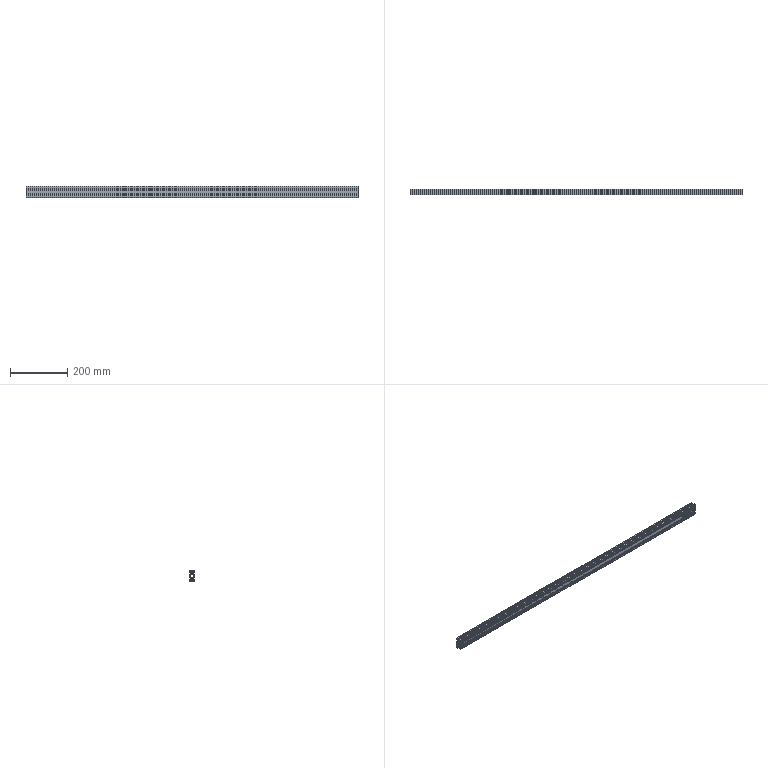Part | STEP file | 1 solid | 212 faces | box 1157 x 20 x 40 mm | volume 344768 mm3 | plane 120 | cylinder 92 | commonest cylinder face diameters 0.6 x68 4 x16 3 x4 5 x4